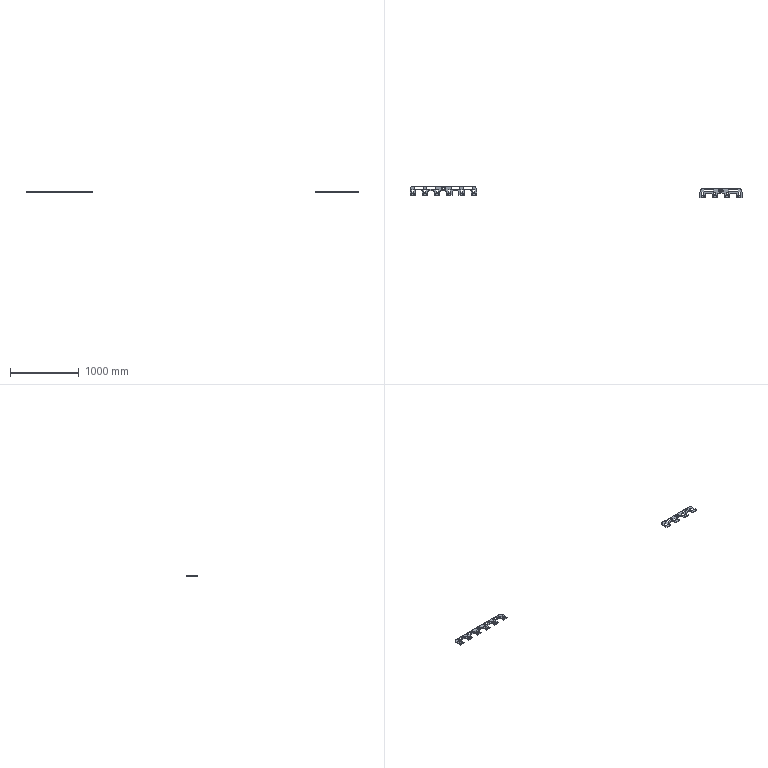Part | 2 solids | 302 faces | box 4825 x 168.213 x 13 mm | volume 1421150 mm3 | cylinder 158 | plane 144 | commonest cylinder face diameters 6 x64 6.5 x40 4.5 x16 8 x16 40 x16 100 x4